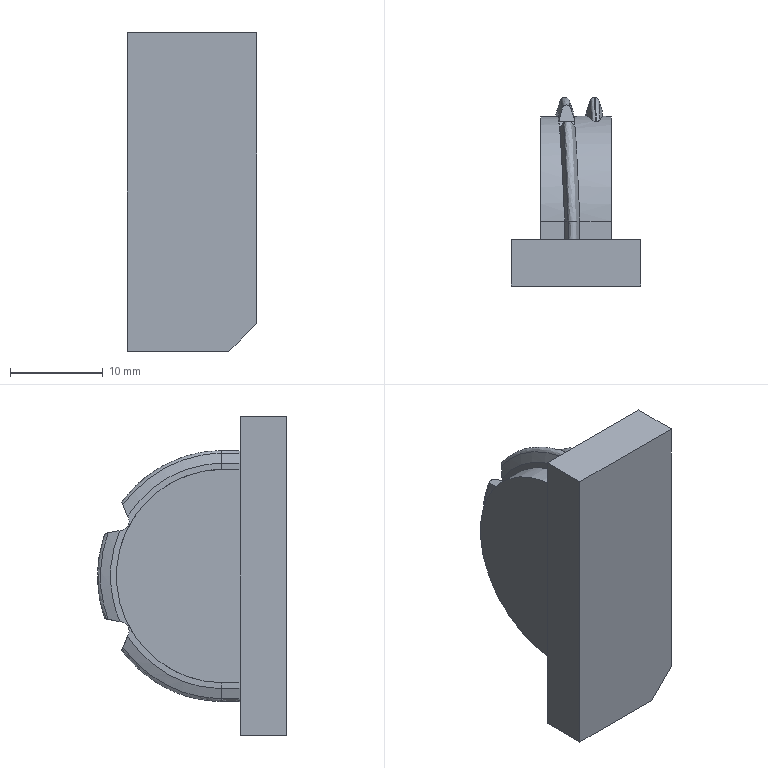NC program | NX | posted with a generic post | part box 13.933 x 20.347 x 34.335 mm
Lines 5575 to 6510 of 105565:
(CAVITY_MILL_COPY , TOOL : D1.5)
N11124 M6
N11126 G54
N11128 G17 G0 G90 X1.692 Y0.818 S2992 M3
N11130 G43 Z3. H0
N11132 Z0.12
N11134 G94 G1 Z-0.08 F1250.
N11136 G2 X0.755 Y0.448 R1.
N11138 G1 X0.701 Y0.456 F2500.
N11140 X0.746 Y0.482
N11142 X0.731 Y0.541
N11144 G3 X0.514 Y0.93 R0.81
N11146 X0.686 Y1.34 R0.81
N11148 G1 X0.706 Y1.478
N11150 G2 X0.134 Y1.019 R1.051
N11152 X-0.965 Y1.454 R1.044
N11154 G3 X-2.133 Y1.836 R1.
N11156 G1 Z0.12
N11158 G0 Z0.3
N11160 G1 X-2.323 Y-0.127 F5000.
N11162 G0 Z0.12
N11164 G1 Z-0.08 F1250.
N11166 G3 X-1.153 Y-0.43 R1.
N11168 G1 X-1.054 Y-0.396 F2500.
N11170 G2 X1.179 Y-0.414 R4.034
N11172 G3 X2.273 Y-0.043 R1.
N11174 G1 Z0.12
N11176 G0 Z0.3
N11178 G1 X-3.308 Y-0.398 F5000.
N11180 G0 Z0.04
N11182 G1 Z-0.16 F1250.
N11184 G3 X-2.096 Y-0.489 R1.
N11186 G2 X-1.871 Y-0.383 R0.913 F2500.
N11188 X1.693 Y-0.166 R6.701
N11190 G1 X1.742 Y-0.178
N11192 G3 X2.87 Y0.296 R1.
N11194 G1 Z0.04
N11196 G0 Z0.22
N11198 G1 X2.017 Y2.102 F5000.
N11200 G0 Z0.04
N11202 G1 Z-0.16 F1250.
N11204 G3 X0.92 Y1.524 R1.
N11206 G2 X0.065 Y0.854 R1.158 F2500.
N11208 G1 X-0.001 Y0.842
N11210 X-1.416 Y1.082
N11212 X-1.488 Y1.114
N11214 G2 X-1.845 Y1.389 R0.943
N11216 G3 X-3.029 Y1.68 R1.
N11218 G1 Z0.04
N11220 G0 Z0.22
N11222 G1 X-3.919 Y-0.571 F5000.
N11224 G0 Z-0.039
N11226 G1 Z-0.239 F1250.
N11228 G3 X-2.693 Y-0.491 R1.
N11230 G2 X-2.182 Y-0.243 R1.043 F2500.
N11232 X2.131 Y-0.093 R10.657
N11234 G3 X3.221 Y0.504 R1.
N11236 G1 Z-0.039
N11238 G0 Z0.14
N11240 G1 X2.103 Y2.452 F5000.
N11242 G0 Z-0.039
N11244 G1 Z-0.239 F1250.
N11246 G3 X1.11 Y1.698 R1.
N11248 G2 X-0.041 Y0.76 R1.244 F2500.
N11250 X-2.124 Y1.033 R6.058
N11252 X-2.554 Y1.319 R0.927
N11254 G3 X-3.743 Y1.58 R1.
N11256 G1 Z-0.039
N11258 G0 Z0.14
N11260 G1 X-4.376 Y-0.693 F5000.
N11262 G0 Z-0.119
N11264 G1 Z-0.319 F1250.
N11266 G3 X-3.155 Y-0.531 R1.
N11268 G2 X-2.617 Y-0.232 R1.08 F2500.
N11270 X1.87 Y0.06 R14.666
N11272 G1 X2.432 Y-0.031
N11274 G3 X3.53 Y0.615 R1.
N11276 G1 Z-0.119
N11278 G0 Z0.061
N11280 G1 X2.276 Y2.331 F5000.
N11282 G0 Z-0.119
N11284 G1 Z-0.319 F1250.
N11286 G3 X1.279 Y1.685 R1.
N11288 G2 X-0.157 Y0.691 R1.534 F2500.
N11290 X-2.494 Y0.896 R13.362
N11292 X-3.096 Y1.272 R1.046
N11294 G3 X-4.29 Y1.565 R1.
N11296 G1 Z-0.119
N11298 G0 Z0.061
N11300 G1 X-4.754 Y-0.666 F5000.
N11302 G0 Z-0.199
N11304 G1 Z-0.399 F1250.
N11306 G3 X-3.529 Y-0.535 R1.
N11308 G2 X-3.118 Y-0.286 R1.073 F2500.
N11310 X-1.247 Y0.072 R7.613
N11312 G1 X0.935 Y0.164
N11314 X1.246 Y0.165
N11316 G2 X2.622 Y0.048 R7.227
N11318 G3 X3.754 Y0.727 R1.
N11320 G1 Z-0.199
N11322 G0 Z-0.019
N11324 G1 X2.379 Y2.546 F5000.
N11326 G0 Z-0.199
N11328 G1 Z-0.399 F1250.
N11330 G3 X1.421 Y1.747 R1.
N11332 G2 X0.667 Y0.842 R1.247 F2500.
N11334 X-0.624 Y0.666 R2.654
N11336 X-3.118 Y0.917 R8.04
N11338 X-3.53 Y1.176 R1.011
N11340 G3 X-4.743 Y1.353 R1.
N11342 G1 Z-0.199
N11344 G0 Z-0.019
N11346 G1 X-5.139 Y-0.97 F5000.
N11348 G0 Z-0.279
N11350 G1 Z-0.479 F1250.
N11352 G3 X-3.922 Y-0.665 R1.
N11354 G2 X-3.133 Y-0.163 R1.337 F2500.
N11356 X-1.386 Y0.091 R13.887
N11358 X2.181 Y0.172 R30.478
N11360 X2.832 Y0.107 R3.536
N11362 G3 X3.978 Y0.788 R1.
N11364 G1 Z-0.279
N11366 G0 Z-0.099
N11368 G1 X2.562 Y2.473 F5000.
N11370 G0 Z-0.279
N11372 G1 Z-0.479 F1250.
N11374 G3 X1.578 Y1.714 R1.
N11376 G2 X0.951 Y0.931 R1.199 F2500.
N11378 X-0.312 Y0.62 R2.721
N11380 G1 X-0.852 Y0.613
N11382 G2 X-3.217 Y0.781 R14.216
N11384 X-3.895 Y1.166 R1.104
N11386 G3 X-5.103 Y1.425 R1.
N11388 G1 Z-0.279
N11390 G0 Z-0.099
N11392 G1 X-5.401 Y-0.794 F5000.
N11394 G0 Z-0.358
N11396 G1 Z-0.558 F1250.
N11398 G3 X-4.176 Y-0.577 R1.
N11400 G2 X-3.614 Y-0.218 R1.209 F2500.
N11402 X-2.338 Y0.028 R6.648
N11404 G1 X-1.559 Y0.1
N11406 X-1.247 Y0.133
N11408 G2 X2.993 Y0.155 R29.622
N11410 G3 X4.035 Y0.932 R1.
N11412 G1 Z-0.358
N11414 G0 Z-0.179
N11416 G1 X2.649 Y2.621 F5000.
N11418 G0 Z-0.358
N11420 G1 Z-0.558 F1250.
N11422 G3 X1.708 Y1.8 R1.
N11424 G2 X0.882 Y0.831 R1.266 F2500.
N11426 X-0.936 Y0.588 R4.522
N11428 X-3.578 Y0.773 R11.454
N11430 X-4.189 Y1.089 R1.105
N11432 G3 X-5.414 Y1.246 R1.
N11434 G1 Z-0.358
N11436 G0 Z-0.179
N11438 G1 X-5.703 Y-1.073 F5000.
N11440 G0 Z-0.438
N11442 G1 Z-0.638 F1250.
N11444 G3 X-4.506 Y-0.708 R1.
N11446 G2 X-3.741 Y-0.177 R1.301 F2500.
N11448 X-2.182 Y0.084 R8.732
N11450 G1 X-1.871 Y0.104
N11452 G2 X2.779 Y0.211 R30.461
N11454 X3.116 Y0.183 R6.338
N11456 G1 X3.213 Y0.182
N11458 G3 X4.23 Y0.972 R1.
N11460 G1 Z-0.438
N11462 G0 Z-0.258
N11464 G1 X2.783 Y2.651 F5000.
N11466 G0 Z-0.438
N11468 G1 Z-0.638 F1250.
N11470 G3 X1.854 Y1.817 R1.
N11472 G2 X0.935 Y0.802 R1.267 F2500.
N11474 X-0.312 Y0.567 R4.759
N11476 G1 X-1.408 Y0.556
N11478 G2 X-3.691 Y0.682 R17.289
N11480 X-4.502 Y1.123 R1.257
N11482 G3 X-5.725 Y1.372 R1.
N11484 G1 Z-0.438
N11486 G0 Z-0.258
N11488 G1 X-5.928 Y-0.77 F5000.
N11490 G0 Z-0.518
N11492 G1 Z-0.718 F1250.
N11494 G3 X-4.698 Y-0.564 R1.
N11496 G2 X-4.053 Y-0.184 R1.24 F2500.
N11498 X-2.055 Y0.125 R14.179
N11500 G1 X-1.559 Y0.166
N11502 G2 X3.369 Y0.22 R37.292
N11504 G3 X4.405 Y1.023 R1.
N11506 G1 Z-0.518
N11508 G0 Z-0.338
N11510 G1 X2.766 Y2.954 F5000.
N11512 G0 Z-0.518
N11514 G1 Z-0.718 F1250.
N11516 G3 X1.961 Y1.997 R1.
N11518 G2 X0.998 Y0.773 R1.297 F2500.
N11520 G1 X-0.001 Y0.556
N11522 G2 X-3.741 Y0.626 R29.64
N11524 X-4.774 Y1.137 R1.444
N11526 G3 X-6.013 Y1.373 R1.
N11528 G1 Z-0.518
N11530 G0 Z-0.338
N11532 G1 X-6.171 Y-0.736 F5000.
N11534 G0 Z-0.598
N11536 G1 Z-0.798 F1250.
N11538 G3 X-4.947 Y-0.56 R1.
N11540 G2 X-4.492 Y-0.27 R1.124 F2500.
N11542 G1 X-4.148 Y-0.154
N11544 G2 X-2.009 Y0.155 R14.38
N11546 G1 X-1.559 Y0.192
N11548 G2 X3.428 Y0.255 R39.321
N11550 G1 X3.523 Y0.252
N11552 G3 X4.556 Y1.066 R1.
N11554 G1 Z-0.598
N11556 G0 Z-0.418
N11558 G1 X2.927 Y2.901 F5000.
N11560 G0 Z-0.598
N11562 G1 Z-0.798 F1250.
N11564 G3 X2.098 Y1.965 R1.
N11566 G2 X1.116 Y0.773 R1.293 F2500.
N11568 X-0.001 Y0.533 R38.117
N11570 X-4.053 Y0.621 R27.841
N11572 G1 X-4.364 Y0.695
N11574 G2 X-4.996 Y1.048 R1.194
N11576 G3 X-6.225 Y1.23 R1.
N11578 G1 Z-0.598
N11580 G0 Z-0.418
N11582 G1 X-6.409 Y-0.97 F5000.
N11584 G0 Z-0.677
N11586 G1 Z-0.877 F1250.
N11588 G3 X-5.197 Y-0.658 R1.
N11590 G2 X-4.376 Y-0.154 R1.307 F2500.
N11592 X-2.806 Y0.101 R11.298
N11594 X3.638 Y0.275 R39.213
N11596 G1 X3.681 Y0.272
N11598 G3 X4.732 Y1.096 R1.
N11600 G1 Z-0.677
N11602 G0 Z-0.498
N11604 G1 X3.064 Y2.874 F5000.
N11606 G0 Z-0.677
N11608 G1 Z-0.877 F1250.
N11610 G3 X2.22 Y1.951 R1.
N11612 G2 X1.235 Y0.773 R1.3 F2500.
N11614 X-0.001 Y0.51 R33.032
N11616 X-4.382 Y0.621 R25.93
N11618 X-5.22 Y1.095 R1.222
N11620 G3 X-6.427 Y1.4 R1.
N11622 G1 Z-0.677
N11624 G0 Z-0.498
N11626 G1 X-6.474 Y-0.841 F5000.
N11628 G0 Z-0.757
N11630 G1 Z-0.957 F1250.
N11632 G3 X-5.27 Y-0.559 R1.
N11634 G2 X-4.581 Y-0.154 R1.121 F2500.
N11636 X-2.182 Y0.191 R17.339
N11638 G1 X-1.559 Y0.245
N11640 G2 X3.428 Y0.316 R39.529
N11642 X3.861 Y0.285 R7.254
N11644 G3 X4.949 Y1.118 R1.
N11646 G1 Z-0.757
N11648 G0 Z-0.577
N11650 G1 X3.261 Y2.754 F5000.
N11652 G0 Z-0.757
N11654 G1 Z-0.957 F1250.
N11656 G3 X2.362 Y1.889 R1.
N11658 G2 X1.69 Y0.934 R1.26 F2500.
N11660 X0.623 Y0.622 R2.922
N11662 X-0.298 Y0.472 R4.012
N11664 X-4.364 Y0.557 R30.823
N11666 X-5.285 Y0.967 R1.486
N11668 G3 X-6.451 Y1.125 R1.
N11670 G1 Z-0.757
N11672 G0 Z-0.577
N11674 G1 X-6.484 Y-0.669 F5000.
N11676 G0 Z-0.837
N11678 G1 Z-1.037 F1250.
N11680 G3 X-5.283 Y-0.444 R1.
N11682 G2 X-4.676 Y-0.125 R0.977 F2500.
N11684 X-0.001 Y0.363 R30.069
N11686 X4.08 Y0.284 R28.956
N11688 G3 X5.159 Y1.137 R1.
N11690 G1 Z-0.837
N11692 G0 Z-0.657
N11694 G1 X3.395 Y2.755 F5000.
N11696 G0 Z-0.837
N11698 G1 Z-1.037 F1250.
N11700 G3 X2.492 Y1.893 R1.
N11702 G2 X1.764 Y0.914 R1.262 F2500.
N11704 G1 X1.455 Y0.773
N11706 X-0.002 Y0.464
N11708 X-0.312 Y0.437
N11710 G2 X-4.676 Y0.561 R30.393
N11712 X-5.291 Y0.882 R0.965
N11714 G3 X-6.49 Y1.116 R1.
N11716 G1 Z-0.837
N11718 G0 Z-0.657
N11720 G1 X-6.504 Y-0.626 F5000.
N11722 G0 Z-0.917
N11724 G1 Z-1.117 F1250.
N11726 G3 X-5.305 Y-0.394 R1.
N11728 G2 X-4.676 Y-0.074 R0.961 F2500.
N11730 X4.19 Y0.31 R37.517
N11732 G3 X5.255 Y1.16 R1.
N11734 G1 Z-0.917
N11736 G0 Z-0.737
N11738 G1 X3.483 Y2.819 F5000.
N11740 G0 Z-0.917
N11742 G1 Z-1.117 F1250.
N11744 G3 X2.6 Y1.936 R1.
N11746 G2 X2.272 Y1.214 R1.273 F2500.
N11748 X1.454 Y0.749 R1.545
N11750 G1 X-0.001 Y0.441
N11752 X-0.312 Y0.411
N11754 G2 X-4.676 Y0.516 R35.736
N11756 X-5.31 Y0.828 R0.937
N11758 G3 X-6.506 Y1.059 R1.
N11760 G1 Z-0.917
N11762 G0 Z0.3
N11764 G1 X3.574 Y2.848 F5000.
N11766 G0 Z-0.997
N11768 G1 Z-1.197 F1250.
N11770 G3 X2.707 Y1.944 R1.
N11772 G2 X2.531 Y1.392 R1.316 F2500.
N11774 X1.558 Y0.748 R1.679
N11776 G1 X-0.007 Y0.417
N11778 G2 X4.239 Y0.346 R37.989
N11780 G3 X5.3 Y1.189 R1.
N11782 G1 Z-0.997
N11784 G0 Z-0.817
N11786 G1 X3.736 Y2.767 F5000.
N11788 G0 Z-1.076
N11790 G1 Z-1.276 F1250.
N11792 G3 X2.83 Y1.907 R1.
N11794 G2 X2.084 Y0.915 R1.275 F2500.
N11796 G1 X1.765 Y0.773
N11798 X0.326 Y0.457
N11800 G2 X4.355 Y0.365 R38.993
N11802 G3 X5.413 Y1.181 R1.
N11804 G1 Z-1.076
N11806 G0 Z-0.897
N11808 G1 X3.819 Y2.821 F5000.
N11810 G0 Z-1.156
N11812 G1 Z-1.356 F1250.
N11814 G3 X2.93 Y1.942 R1.
N11816 G2 X2.569 Y1.189 R1.283 F2500.
N11818 X1.866 Y0.773 R1.596
N11820 G1 X0.61 Y0.492
N11822 G2 X4.423 Y0.389 R39.468
N11824 G3 X5.478 Y1.187 R1.
N11826 G1 Z-1.156
N11828 G0 Z-0.976
N11830 G1 X3.867 Y2.922 F5000.
N11832 G0 Z-1.236
N11834 G1 Z-1.436 F1250.
N11836 G3 X3.027 Y1.991 R1.
N11838 G2 X2.847 Y1.392 R1.338 F2500.
N11840 X1.87 Y0.751 R1.695
N11842 G1 X0.864 Y0.523
N11844 G2 X4.493 Y0.411 R39.352
N11846 G3 X5.546 Y1.19 R1.
N11848 G1 Z-1.236
N11850 G0 Z-1.056
N11852 G1 X4.041 Y2.824 F5000.
N11854 G0 Z-1.316
N11856 G1 Z-1.516 F1250.
N11858 G3 X3.151 Y1.946 R1.
N11860 G2 X2.383 Y0.916 R1.283 F2500.
N11862 G1 X2.05 Y0.773
N11864 X1.11 Y0.555
N11866 G2 X4.579 Y0.43 R39.892
N11868 G3 X5.628 Y1.18 R1.
N11870 G1 Z-1.316
N11872 G0 Z-1.136
N11874 G1 X4.09 Y2.914 F5000.
N11876 G0 Z-1.395
N11878 G1 Z-1.595 F1250.
N11880 G3 X3.238 Y1.998 R1.
N11882 G2 X2.493 Y0.913 R1.304 F2500.
N11884 X1.324 Y0.583 R5.381
N11886 X4.627 Y0.452 R38.859
N11888 G3 X5.675 Y1.185 R1.
N11890 G1 Z-1.395
N11892 G0 Z-1.216
N11894 G1 X4.171 Y2.934 F5000.
N11896 G0 Z-1.475
N11898 G1 Z-1.675 F1250.
N11900 G3 X3.325 Y2.011 R1.
N11902 G2 X2.493 Y0.869 R1.32 F2500.
N11904 X1.439 Y0.589 R6.841
N11906 X4.665 Y0.476 R28.827
N11908 G3 X5.717 Y1.193 R1.
N11910 G1 Z-1.475
N11912 G0 Z-1.295
N11914 G1 X4.32 Y2.842 F5000.
N11916 G0 Z-1.555
N11918 G1 Z-1.755 F1250.
N11920 G3 X3.436 Y1.955 R1.
N11922 G2 X2.493 Y0.835 R1.311 F2500.
N11924 G1 X1.651 Y0.597
N11926 G2 X4.736 Y0.488 R20.935
N11928 G3 X5.797 Y1.174 R1.
N11930 G1 Z-1.555
N11932 G0 Z-1.375
N11934 G1 X4.407 Y2.859 F5000.
N11936 G0 Z-1.635
N11938 G1 Z-1.835 F1250.
N11940 G3 X3.526 Y1.97 R1.
N11942 G2 X2.697 Y0.889 R1.306 F2500.
N11944 X1.655 Y0.598 R5.685
N11946 X4.774 Y0.513 R17.963
N11948 G3 X5.835 Y1.185 R1.
N11950 G1 Z-1.635
N11952 G0 Z-1.455
N11954 G1 X4.463 Y2.942 F5000.
N11956 G0 Z-1.714
N11958 G1 Z-1.914 F1250.
N11960 G3 X3.614 Y2.021 R1.
N11962 G2 X2.805 Y0.892 R1.321 F2500.
N11964 X1.772 Y0.605 R4.875
N11966 X4.821 Y0.535 R16.579
N11968 G3 X5.877 Y1.191 R1.
N11970 G1 Z-1.714
N11972 G0 Z-1.535
N11974 G1 X4.583 Y2.887 F5000.
N11976 G0 Z-1.794
N11978 G1 Z-1.994 F1250.
N11980 G3 X3.712 Y1.987 R1.
N11982 G2 X2.805 Y0.854 R1.318 F2500.
N11984 G1 X1.95 Y0.611
N11986 G2 X4.866 Y0.558 R14.601
N11988 G3 X5.919 Y1.198 R1.
N11990 G1 Z-1.794
N11992 G0 Z-1.614
N11994 G1 X4.678 Y2.876 F5000.
N11996 G0 Z-1.874
N11998 G1 Z-2.074 F1250.
N12000 G3 X3.798 Y1.985 R1.
N12002 G2 X3.116 Y0.965 R1.313 F2500.
N12004 X1.975 Y0.615 R4.103
N12006 X4.895 Y0.581 R15.168
N12008 G3 X5.937 Y1.219 R1.
N12010 G1 Z-1.874
N12012 G0 Z-1.694
N12014 G1 X4.76 Y2.887 F5000.
N12016 G0 Z-1.954
N12018 G1 Z-2.154 F1250.
N12020 G3 X3.886 Y1.992 R1.
N12022 G2 X3.116 Y0.928 R1.302 F2500.
N12024 X2.075 Y0.62 R4.487
N12026 X4.907 Y0.613 R16.485
N12028 G1 X4.92 Y0.611
N12030 G3 X5.956 Y1.246 R1.
N12032 G1 Z-1.954
N12034 G0 Z-1.774
N12036 G1 X4.852 Y2.818 F5000.
N12038 G0 Z-2.033
N12040 G1 Z-2.233 F1250.
N12042 G3 X3.966 Y1.986 R1.
N12044 G2 X2.668 Y0.747 R1.494 F2500.
N12046 G1 Y0.645
N12048 G2 X4.964 Y0.627 R11.273
N12050 G3 X6. Y1.244 R1.
N12052 G1 Z-2.033
N12054 G0 Z-1.854
N12056 G1 X4.928 Y2.884 F5000.
N12058 G0 Z-2.113
N12060 G1 Z-2.313 F1250.
N12062 G3 X4.048 Y1.991 R1.
N12064 G2 X3.105 Y0.849 R1.333 F2500.
N12066 G1 Y0.664
N12068 G2 X4.987 Y0.652 R10.087
N12070 G1 X5.029 Y0.644
N12072 G3 X6.116 Y1.187 R1.
N12074 G1 Z-2.113
N12076 G0 Z-1.933
N12078 G1 X5.023 Y2.852 F5000.
N12080 G0 Z-2.193
N12082 G1 Z-2.393 F1250.
N12084 G3 X4.128 Y1.976 R1.
N12086 G2 X3.469 Y0.985 R1.32 F2500.
N12088 G1 Y0.68
N12090 G2 X4.987 Y0.678 R7.303
N12092 G1 X5.038 Y0.67
N12094 G3 X6.12 Y1.223 R1.
N12096 G1 Z-2.193
N12098 G0 Z-2.013
N12100 G1 X5.104 Y2.847 F5000.
N12102 G0 Z-2.273
N12104 G1 Z-2.473 F1250.
N12106 G3 X4.204 Y1.974 R1.
N12108 G2 X3.786 Y1.162 R1.327 F2500.
N12110 G1 Y0.694
N12112 G2 X4.987 Y0.705 R8.093
N12114 G1 X5.073 Y0.691
N12116 G3 X6.167 Y1.219 R1.
N12118 G1 Z-2.273
N12120 G0 Z-2.093
N12122 G1 X5.181 Y2.846 F5000.
N12124 G0 Z-2.353
N12126 G1 Z-2.553 F1250.
N12128 G3 X4.279 Y1.971 R1.
N12130 G2 X4.071 Y1.393 R1.385 F2500.
N12132 G1 Y0.707
N12134 X4.893 Y0.727
N12136 G2 X5.115 Y0.705 R0.898
N12138 G3 X6.219 Y1.208 R1.
N12140 G1 Z-2.353
N12142 G0 Z-2.173
N12144 G1 X5.331 Y3.052 F5000.
N12146 G0 Z-2.432
N12148 G1 Z-2.632 F1250.
N12150 G3 X4.331 Y2.052 R1.
N12152 G1 Y0.719 F2500.
N12154 X4.913 Y0.733
N12156 G2 X5.148 Y0.707 R0.894
N12158 G3 X6.261 Y1.192 R1.
N12160 G1 Z-2.432
N12162 G0 Z-2.253
N12164 G1 X7.692 Y-3.064 F5000.
N12166 G0 Z-2.512
N12168 G1 Z-2.712 F1250.
N12170 G3 X7.34 Y-1.91 R1.
N12172 G2 X6.995 Y-1.235 R0.833 F2500.
N12174 G1 Y-0.546
N12176 G2 X7.345 Y0.136 R0.839
N12178 G3 X7.702 Y1.288 R1.
N12180 G1 Z-2.512
N12182 G0 Z-2.332
N12184 G1 X5.667 Y1.783 F5000.
N12186 G0 Z-2.512
N12188 G1 Z-2.712 F1250.
N12190 G3 X5.628 Y0.424 R1.
N12192 G2 X5.845 Y-0.153 R0.875 F2500.
N12194 G1 Y-1.8
N12196 G2 X5.707 Y-2.278 R0.916
N12198 G3 X5.827 Y-3.488 R1.
N12200 G1 Z-2.512
N12202 G0 Z3.
N12204 X5.572 Y2.878
N12206 Z-2.512
N12208 G1 Z-2.712 F1250.
N12210 G3 X4.572 Y1.878 R1.
N12212 G1 Y0.73 F2500.
N12214 G2 X5.276 Y0.667 R1.331
N12216 G1 X5.313 Y0.652
N12218 G3 X6.594 Y1.111 R1.
N12220 G1 Z-2.512
N12222 G0 Z3.
N12224 X-6.525 Y-0.587
N12226 Z-0.997
N12228 G1 Z-1.197 F1250.
N12230 G3 X-5.332 Y-0.357 R1.
N12232 G2 X-4.8 Y-0.066 R0.904 F2500.
N12234 X-0.866 Y0.372 R41.268
N12236 X-4.676 Y0.478 R36.968
N12238 X-5.337 Y0.797 R0.923
N12240 G3 X-6.528 Y1.044 R1.
N12242 G1 Z-0.997
N12244 G0 Z-0.817
N12246 G1 X-6.551 Y-0.617 F5000.
N12248 G0 Z-1.076
N12250 G1 Z-1.276 F1250.
N12252 G3 X-5.367 Y-0.35 R1.
N12254 G2 X-4.805 Y-0.036 R0.9 F2500.
N12256 G1 X-4.364 Y0.027
N12258 X-2.182 Y0.294
N12260 X-1.691 Y0.338
N12262 G2 X-4.676 Y0.448 R34.853
N12264 X-5.372 Y0.798 R0.935
N12266 G3 X-6.555 Y1.088 R1.
N12268 G1 Z-1.076
N12270 G0 Z-0.897
N12272 G1 X-6.576 Y-0.656 F5000.
N12274 G0 Z-1.156
N12276 G1 Z-1.356 F1250.
N12278 G3 X-5.403 Y-0.36 R1.
N12280 G2 X-4.988 Y-0.074 R0.868 F2500.
N12282 G1 X-4.676 Y0.008
N12284 X-4.364 Y0.051
N12286 X-2.261 Y0.313
N12288 G2 X-4.676 Y0.423 R33.753
N12290 X-5.4 Y0.789 R0.934
N12292 G3 X-6.576 Y1.105 R1.
N12294 G1 Z-1.156
N12296 G0 Z-0.976
N12298 G1 X-6.59 Y-0.62 F5000.
N12300 G0 Z-1.236
N12302 G1 Z-1.436 F1250.
N12304 G3 X-5.414 Y-0.332 R1.
N12306 G2 X-4.988 Y-0.046 R0.869 F2500.
N12308 G1 X-4.676 Y0.032
N12310 X-2.697 Y0.293
N12312 X-4.364 Y0.373
N12314 X-4.676 Y0.397
N12316 G2 X-5.416 Y0.761 R0.93
N12318 G3 X-6.592 Y1.077 R1.
N12320 G1 Z-1.236
N12322 G0 Z-1.056
N12324 G1 X-6.607 Y-0.608 F5000.
N12326 G0 Z-1.316
N12328 G1 Z-1.516 F1250.
N12330 G3 X-5.433 Y-0.313 R1.
N12332 G2 X-4.988 Y-0.019 R0.869 F2500.
N12334 G1 X-4.676 Y0.055
N12336 X-3.061 Y0.276
N12338 X-4.364 Y0.346
N12340 X-4.786 Y0.38
N12342 G2 X-5.432 Y0.729 R0.91
N12344 G3 X-6.607 Y1.038 R1.
N12346 G1 Z-1.316
N12348 G0 Z-1.136
N12350 G1 X-6.624 Y-0.602 F5000.
N12352 G0 Z-1.395
N12354 G1 Z-1.595 F1250.
N12356 G3 X-5.452 Y-0.297 R1.
N12358 G2 X-4.988 Y0.008 R0.874 F2500.
N12360 G1 X-4.676 Y0.079
N12362 X-3.391 Y0.262
N12364 X-4.786 Y0.352
N12366 G2 X-5.452 Y0.709 R0.912
N12368 G3 X-6.624 Y1.027 R1.
N12370 G1 Z-1.395
N12372 G0 Z-1.216
N12374 G1 X-6.642 Y-0.602 F5000.
N12376 G0 Z-1.475
N12378 G1 Z-1.675 F1250.
N12380 G3 X-5.472 Y-0.283 R1.
N12382 G2 X-4.988 Y0.036 R0.882 F2500.
N12384 X-3.671 Y0.249 R14.075
N12386 G1 X-4.81 Y0.329
N12388 G2 X-5.471 Y0.687 R0.908
N12390 G3 X-6.641 Y1.012 R1.
N12392 G1 Z-1.475
N12394 G0 Z-1.295
N12396 G1 X-6.659 Y-0.602 F5000.
N12398 G0 Z-1.555
N12400 G1 Z-1.755 F1250.
N12402 G3 X-5.493 Y-0.27 R1.
N12404 G2 X-4.988 Y0.063 R0.891 F2500.
N12406 G1 X-3.935 Y0.238
N12408 X-4.862 Y0.323
N12410 G2 X-5.492 Y0.676 R0.889
N12412 G3 X-6.659 Y1.006 R1.
N12414 G1 Z-1.555
N12416 G0 Z-1.375
N12418 G1 X-6.678 Y-0.621 F5000.
N12420 G0 Z-1.635
N12422 G1 Z-1.835 F1250.
N12424 G3 X-5.518 Y-0.264 R1.
N12426 G2 X-4.988 Y0.09 R0.9 F2500.
N12428 G1 X-4.173 Y0.227
N12430 X-4.883 Y0.297
N12432 G2 X-5.513 Y0.655 R0.89
N12434 G3 X-6.676 Y0.996 R1.
N12436 G1 Z-1.635
N12438 G0 Z-1.455
N12440 G1 X-6.693 Y-0.6 F5000.
N12442 G0 Z-1.714
N12444 G1 Z-1.914 F1250.
N12446 G3 X-5.532 Y-0.243 R1.
N12448 G2 X-4.988 Y0.117 R0.909 F2500.
N12450 G1 X-4.399 Y0.218
N12452 X-4.892 Y0.27
N12454 G2 X-5.53 Y0.639 R0.903
N12456 G3 X-6.693 Y0.99 R1.
N12458 G1 Z-1.714
N12460 G0 Z-1.535
N12462 G1 X-6.71 Y-0.596 F5000.
N12464 G0 Z-1.794
N12466 G1 Z-1.994 F1250.
N12468 G3 X-5.551 Y-0.228 R1.
N12470 G2 X-4.988 Y0.145 R0.917 F2500.
N12472 G1 X-4.607 Y0.21
N12474 G2 X-5.553 Y0.645 R0.988
N12476 G3 X-6.712 Y1.038 R1.
N12478 G1 Z-1.794
N12480 G0 Z-1.614
N12482 G1 X-6.727 Y-0.604 F5000.
N12484 G0 Z-1.874
N12486 G1 Z-2.074 F1250.
N12488 G3 X-5.571 Y-0.217 R1.
N12490 G2 X-4.828 Y0.198 R0.944 F2500.
N12492 X-5.567 Y0.602 R0.934
N12494 G3 X-6.726 Y0.976 R1.
N12496 G1 Z-1.874
N12498 G0 Z-1.694
N12500 G1 X-6.743 Y-0.577 F5000.
N12502 G0 Z-1.954
N12504 G1 Z-2.154 F1250.
N12506 G3 X-5.589 Y-0.194 R1.
N12508 G2 X-4.971 Y0.196 R0.917 F2500.
N12510 X-5.585 Y0.578 R0.913
N12512 G3 X-6.742 Y0.95 R1.
N12514 G1 Z-1.954
N12516 G0 Z-1.774
N12518 G1 X-6.759 Y-0.555 F5000.
N12520 G0 Z-2.033
N12522 G1 Z-2.233 F1250.
N12524 G3 X-5.607 Y-0.173 R1.
N12526 G2 X-5.07 Y0.194 R0.895 F2500.
N12528 X-5.603 Y0.557 R0.898
N12530 G3 X-6.758 Y0.931 R1.
N12532 G1 Z-2.033
N12534 G0 Z-1.854
N12536 G1 X-6.776 Y-0.556 F5000.
N12538 G0 Z-2.113
N12540 G1 Z-2.313 F1250.
N12542 G3 X-5.628 Y-0.162 R1.
N12544 G2 X-5.169 Y0.19 R0.896 F2500.
N12546 X-5.628 Y0.547 R0.908
N12548 G3 X-6.776 Y0.946 R1.
N12550 G1 Z-2.113
N12552 G0 Z-1.933
N12554 G1 X-6.792 Y-0.559 F5000.
N12556 G0 Z-2.193
N12558 G1 Z-2.393 F1250.
N12560 G3 X-5.648 Y-0.148 R1.
N12562 G2 X-5.253 Y0.19 R0.915 F2500.
N12564 X-5.647 Y0.528 R0.913
N12566 G3 X-6.792 Y0.936 R1.
N12568 G1 Z-2.193
N12570 G0 Z-2.013
N12572 G1 X-6.809 Y-0.561 F5000.
N12574 G0 Z-2.273
N12576 G1 Z-2.473 F1250.
N12578 G3 X-5.67 Y-0.137 R1.
N12580 G2 X-5.317 Y0.187 R0.907 F2500.
N12582 X-5.668 Y0.515 R0.93
N12584 G3 X-6.808 Y0.942 R1.
N12586 G1 Z-2.273
N12588 G0 Z-2.093
N12590 G1 X-6.824 Y-0.558 F5000.
N12592 G0 Z-2.353
N12594 G1 Z-2.553 F1250.
N12596 G3 X-5.69 Y-0.124 R1.
N12598 G2 X-5.363 Y0.191 R0.91 F2500.
N12600 X-5.688 Y0.501 R0.906
N12602 G3 X-6.824 Y0.929 R1.
N12604 G1 Z-2.353
N12606 G0 Z-2.173
N12608 G1 X-6.84 Y-0.565 F5000.
N12610 G0 Z-2.432
N12612 G1 Z-2.632 F1250.
N12614 G3 X-5.707 Y-0.126 R1.
N12616 G2 X-5.385 Y0.188 R0.911 F2500.
N12618 X-5.703 Y0.492 R0.897
N12620 G3 X-6.84 Y0.918 R1.
N12622 G1 Z-2.432
N12624 G0 Z-2.253
N12626 G1 X-9.836 Y-0.993 F5000.
N12628 G0 Z-2.512
N12630 G1 Z-2.712 F1250.
N12632 G3 X-8.616 Y-0.752 R1.
N12634 G2 X-7.912 Y-0.348 R1.202 F2500.
N12636 X-7.006 Y-1.183 R0.866
N12638 G1 Y-1.868
N12640 G2 X-7.38 Y-2.532 R0.87
N12642 G3 X-7.756 Y-3.683 R1.
N12644 G1 Z-2.512
N12646 G0 Z-2.332
N12648 G1 X-5.714 Y-3.975 F5000.
N12650 G0 Z-2.512
N12652 G1 Z-2.712 F1250.
N12654 G3 X-5.686 Y-2.762 R1.
N12656 G2 X-5.856 Y-2.238 R0.892 F2500.
N12658 G1 Y-0.6
N12660 G2 X-5.405 Y0.184 R0.907
N12662 X-5.856 Y0.967 R0.903
N12664 G1 Y2.599
N12666 G2 X-5.725 Y3.065 R0.917
N12668 G3 X-5.862 Y4.274 R1.
N12670 G1 Z-2.512
N12672 G0 Z-2.332
N12674 G1 X-7.792 Y3.805 F5000.
N12676 G0 Z-2.512
N12678 G1 Z-2.712 F1250.
N12680 G3 X-7.371 Y2.676 R1.
N12682 G2 X-7.006 Y2.015 R0.79 F2500.
N12684 G1 Y1.335
N12686 G2 X-7.16 Y0.938 R0.914
N12688 G1 X-6.632 Y0.129
N12690 X-7.16 Y0.938
N12692 G2 X-8.585 Y0.837 R0.914
N12694 G3 X-9.782 Y1.047 R1.
N12696 G1 Z-2.512
N12698 G0 Z3.
N12700 X-3.949 Y4.551
N12702 Z-1.954
N12704 G1 Z-2.154 F1250.
N12706 G3 X-2.905 Y3.629 R1.
N12708 G2 X-2.097 Y3.648 R16.31 F2500.
N12710 G1 Y3.816
N12712 G2 X-2.011 Y4.145 R0.919
N12714 G3 X-2.267 Y5.334 R1.
N12716 G1 Z-1.954
N12718 G0 Z-1.774
N12720 G1 X-4.642 Y4.48 F5000.
N12722 G0 Z-2.033
N12724 G1 Z-2.233 F1250.
N12726 G3 X-3.576 Y3.585 R1.
N12728 G2 X-2.679 Y3.623 R15.194 F2500.
N12730 G1 Y3.827
N12732 G2 X-2.622 Y4.12 R0.78
N12734 G3 X-2.928 Y5.279 R1.
N12736 G1 Z-2.033
N12738 G0 Z-1.854
N12740 G1 X-5.079 Y4.437 F5000.
N12742 G0 Z-2.113
N12744 G1 Z-2.313 F1250.
N12746 G3 X-4.006 Y3.556 R1.
N12748 G2 X-3.116 Y3.597 R12.792 F2500.
N12750 G1 Y3.82
N12752 G2 X-3.071 Y4.089 R0.819
N12754 G3 X-3.44 Y5.235 R1.
N12756 G1 Z-2.113
N12758 G0 Z-1.933
N12760 G1 X-5.412 Y4.391 F5000.
N12762 G0 Z-2.193
N12764 G1 Z-2.393 F1250.
N12766 G3 X-4.334 Y3.537 R1.
N12768 G2 X-3.48 Y3.583 R12.32 F2500.
N12770 G1 Y3.832
N12772 G2 X-3.442 Y4.073 R0.785
N12774 G3 X-3.832 Y5.208 R1.
N12776 G1 Z-2.193
N12778 G0 Z-2.013
N12780 G1 X-5.725 Y4.293 F5000.
N12782 G0 Z-2.273
N12784 G1 Z-2.473 F1250.
N12786 G3 X-4.697 Y3.519 R1.
N12788 G1 X-3.797 Y3.567 F2500.
N12790 Y3.832
N12792 G2 X-3.754 Y4.091 R0.789
N12794 G3 X-4.121 Y5.234 R1.
N12796 G1 Z-2.273
N12798 G0 Z-2.093
N12800 G1 X-5.869 Y4.238 F5000.
N12802 G0 Z-2.353
N12804 G1 Z-2.553 F1250.
N12806 G3 X-4.853 Y3.513 R1.
N12808 G1 X-4.082 Y3.555 F2500.
N12810 Y3.816
N12812 G2 X-3.988 Y4.121 R1.073
N12814 G3 X-4.249 Y5.325 R1.
N12816 G1 Z-2.353
N12818 G0 Z-2.173
N12820 G1 X-6.1 Y4.104 F5000.
N12822 G0 Z-2.432
N12824 G1 Z-2.632 F1250.
N12826 G3 X-5.043 Y3.502 R1.
N12828 G1 X-4.988 Y3.507 F2500.
N12830 X-4.343 Y3.542
N12832 Y3.816
N12834 G2 X-4.266 Y4.101 R1.036
N12836 G3 X-4.574 Y5.29 R1.
N12838 G1 Z-2.432
N12840 G0 Z-2.253
N12842 G1 X-6.169 Y4.064 F5000.
N12844 G0 Z-2.512
N12846 G1 Z-2.712 F1250.
N12848 G3 X-5.093 Y3.497 R1.
N12850 G1 X-4.988 Y3.509 F2500.
N12852 X-4.583 Y3.536
N12854 Y3.816
N12856 G2 X-4.531 Y4.03 R1.052
N12858 G3 X-4.916 Y5.198 R1.
N12860 G1 Z-2.512
N12862 G0 Z-2.332
N12864 G1 X-6.362 Y3.917 F5000.
N12866 G0 Z-2.592
N12868 G1 Z-2.792 F1250.
N12870 G3 X-5.23 Y3.458 R1.
N12872 G1 X-5.122 Y3.481 F2500.
N12874 X-4.808 Y3.528
N12876 Y3.816
N12878 X-4.77 Y3.987
N12880 G3 X-5.204 Y5.138 R1.
N12882 G1 Z-2.592
N12884 G0 Z3.
N12886 X2.526 Y5.108
N12888 Z-1.954
N12890 G1 Z-2.154 F1250.
N12892 G3 X2.057 Y3.986 R1.
N12894 G1 X2.085 Y3.816 F2500.
N12896 Y3.563
N12898 G2 X2.689 Y3.453 R3.69
N12900 G3 X3.871 Y4.031 R1.
N12902 G1 Z-1.954
N12904 G0 Z-1.774
N12906 G1 X3.334 Y4.865 F5000.
N12908 G0 Z-2.033
N12910 G1 Z-2.233 F1250.
N12912 G3 X2.667 Y3.868 R1.
N12914 G1 X2.668 Y3.827 F2500.
N12916 Y3.485
N12918 G2 X3.063 Y3.394 R1.423
N12920 G3 X4.262 Y3.779 R1.
N12922 G1 Z-2.033
N12924 G0 Z-1.854
N12926 G1 X3.857 Y4.741 F5000.
N12928 G0 Z-2.113
N12930 G1 Z-2.313 F1250.
N12932 G3 X3.105 Y3.772 R1.
N12934 G1 Y3.403 F2500.
N12936 G2 X3.401 Y3.273 R1.333
N12938 G3 X4.642 Y3.451 R1.
N12940 G1 Z-2.113
N12942 G0 Z-1.933
N12944 G1 X4.292 Y4.599 F5000.
N12946 G0 Z-2.193
N12948 G1 Z-2.393 F1250.
N12950 G3 X3.469 Y3.615 R1.
N12952 G1 Y3.281 F2500.
N12954 G2 X3.664 Y3.145 R1.32
N12956 G3 X4.917 Y3.12 R1.
N12958 G1 Z-2.193
N12960 G0 Z-2.013
N12962 G1 X4.716 Y4.321 F5000.
N12964 G0 Z-2.273
N12966 G1 Z-2.473 F1250.
N12968 G3 X3.786 Y3.323 R1.
N12970 G1 Y3.114 F2500.
N12972 X3.88 Y3.018
N12974 G3 X5.116 Y2.807 R1.
N12976 G1 Z-2.273
N12978 G0 Z-2.093
N12980 G1 X5.061 Y3.977 F5000.
N12982 G0 Z-2.353
N12984 G1 Z-2.553 F1250.
N12986 G3 X4.071 Y2.977 R1.
N12988 G1 Y2.884 F2500.